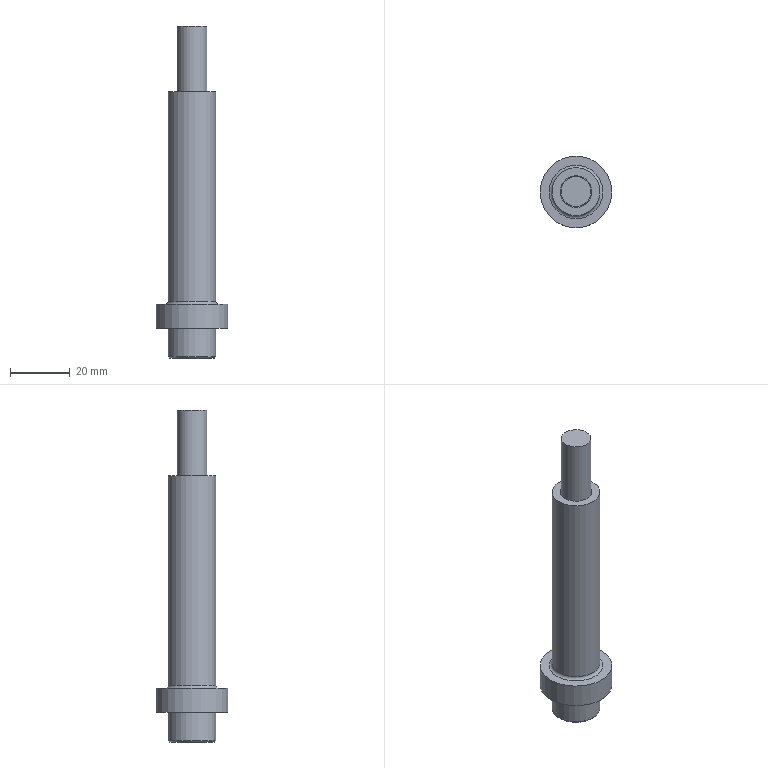Part | STEP file | 1_id286_x_t | 1 solid | 252 faces | box 24 x 24 x 111 mm | volume 20570 mm3 | plane 125 | other 119 | cylinder 5 | cone 2 | torus 1 | commonest cylinder face diameters 16 x2 10 x1 10.6 x1 24 x1